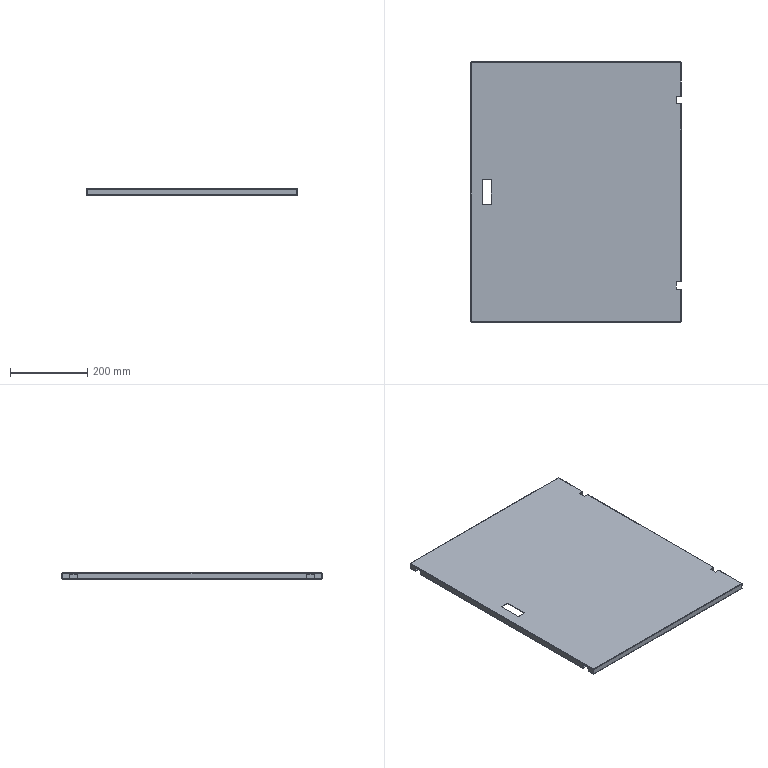Part | SolidWorks | 1 solid | 142 faces | box 545.5 x 674 x 16.5 mm | volume 628405 mm3 | plane 94 | cylinder 32 | spline 16 | commonest cylinder face diameters 0.2 x14 3.2 x14 6 x4